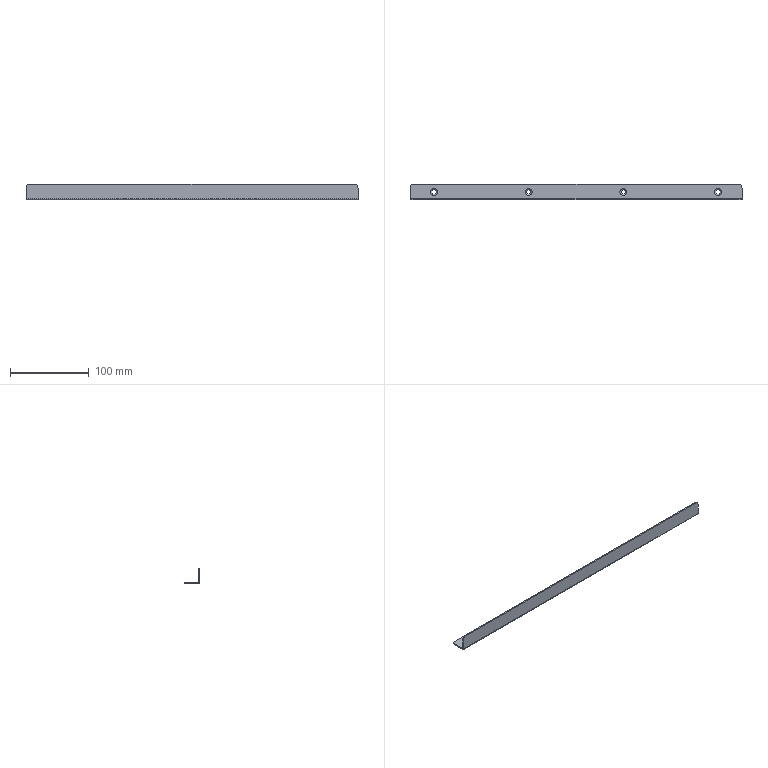Part | SolidWorks | features Chamfer 1, EdgeFlange 1, Fillet 1, FlatPattern 1, ICE 1, LPattern 1, SMBaseFlange 1, SheetMetal 1 | 1 solid | 26 faces | box 421 x 20 x 20 mm | volume 23768 mm3 | plane 12 | cone 8 | cylinder 6 | commonest cylinder face diameters 10 x4 0.4 x1 3.4 x1
STEP:
#1=CARTESIAN_POINT('',(-182.9,0.,-1.5));
#2=VERTEX_POINT('',#1);
#3=CARTESIAN_POINT('',(-177.1,0.,-1.5));
#4=VERTEX_POINT('',#3);
#5=CARTESIAN_POINT('',(-180.,0.,-1.5));
#6=DIRECTION('',(0.,0.,1.));
#7=DIRECTION('',(1.,0.,0.));
#8=AXIS2_PLACEMENT_3D('',#5,#6,#7);
#9=CIRCLE('',#8,2.9);
#10=EDGE_CURVE('',#2,#4,#9,.T.);
#11=ORIENTED_EDGE('',*,*,#10,.F.);
#12=CARTESIAN_POINT('',(-184.4,0.,0.));
#13=VERTEX_POINT('',#12);
#14=CARTESIAN_POINT('',(-182.9,0.,-1.5));
#15=DIRECTION('',(-0.7071,0.,0.7071));
#16=VECTOR('',#15,1000.);
#17=LINE('',#14,#16);
#18=EDGE_CURVE('',#2,#13,#17,.T.);
#19=ORIENTED_EDGE('',*,*,#18,.T.);
#20=CARTESIAN_POINT('',(-175.6,0.,0.));
#21=VERTEX_POINT('',#20);
#22=CARTESIAN_POINT('',(-180.,0.,0.));
#23=DIRECTION('',(0.,0.,-1.));
#24=DIRECTION('',(1.,0.,0.));
#25=AXIS2_PLACEMENT_3D('',#22,#23,#24);
#26=CIRCLE('',#25,4.4);
#27=EDGE_CURVE('',#21,#13,#26,.T.);
#28=ORIENTED_EDGE('',*,*,#27,.F.);
#29=CARTESIAN_POINT('',(-177.1,0.,-1.5));
#30=DIRECTION('',(0.7071,0.,0.7071));
#31=VECTOR('',#30,1000.);
#32=LINE('',#29,#31);
#33=EDGE_CURVE('',#4,#21,#32,.T.);
#34=ORIENTED_EDGE('',*,*,#33,.F.);
#35=EDGE_LOOP('',(#11,#19,#28,#34));
#36=FACE_OUTER_BOUND('',#35,.T.);
#37=CARTESIAN_POINT('',(-180.,0.,-1.5));
#38=DIRECTION('',(0.,0.,1.));
#39=DIRECTION('',(1.,0.,0.));
#40=AXIS2_PLACEMENT_3D('',#37,#38,#39);
#41=CONICAL_SURFACE('',#40,2.9,0.7854);
#42=ADVANCED_FACE('',(#36),#41,.F.);
#43=CARTESIAN_POINT('',(-62.9,0.,-1.5));
#44=VERTEX_POINT('',#43);
#45=CARTESIAN_POINT('',(-57.1,0.,-1.5));
#46=VERTEX_POINT('',#45);
#47=CARTESIAN_POINT('',(-60.,0.,-1.5));
#48=DIRECTION('',(0.,0.,1.));
#49=DIRECTION('',(1.,0.,0.));
#50=AXIS2_PLACEMENT_3D('',#47,#48,#49);
#51=CIRCLE('',#50,2.9);
#52=EDGE_CURVE('',#44,#46,#51,.T.);
#53=ORIENTED_EDGE('',*,*,#52,.F.);
#54=CARTESIAN_POINT('',(-64.4,0.,0.));
#55=VERTEX_POINT('',#54);
#56=CARTESIAN_POINT('',(-62.9,0.,-1.5));
#57=DIRECTION('',(-0.7071,0.,0.7071));
#58=VECTOR('',#57,1000.);
#59=LINE('',#56,#58);
#60=EDGE_CURVE('',#44,#55,#59,.T.);
#61=ORIENTED_EDGE('',*,*,#60,.T.);
#62=CARTESIAN_POINT('',(-55.6,0.,0.));
#63=VERTEX_POINT('',#62);
#64=CARTESIAN_POINT('',(-60.,0.,0.));
#65=DIRECTION('',(0.,0.,-1.));
#66=DIRECTION('',(1.,0.,0.));
#67=AXIS2_PLACEMENT_3D('',#64,#65,#66);
#68=CIRCLE('',#67,4.4);
#69=EDGE_CURVE('',#63,#55,#68,.T.);
#70=ORIENTED_EDGE('',*,*,#69,.F.);
#71=CARTESIAN_POINT('',(-57.1,0.,-1.5));
#72=DIRECTION('',(0.7071,0.,0.7071));
#73=VECTOR('',#72,1000.);
#74=LINE('',#71,#73);
#75=EDGE_CURVE('',#46,#63,#74,.T.);
#76=ORIENTED_EDGE('',*,*,#75,.F.);
#77=EDGE_LOOP('',(#53,#61,#70,#76));
#78=FACE_OUTER_BOUND('',#77,.T.);
#79=CARTESIAN_POINT('',(-60.,0.,-1.5));
#80=DIRECTION('',(0.,0.,1.));
#81=DIRECTION('',(1.,0.,0.));
#82=AXIS2_PLACEMENT_3D('',#79,#80,#81);
#83=CONICAL_SURFACE('',#82,2.9,0.7854);
#84=ADVANCED_FACE('',(#78),#83,.F.);
#85=CARTESIAN_POINT('',(57.1,0.,-1.5));
#86=VERTEX_POINT('',#85);
#87=CARTESIAN_POINT('',(62.9,0.,-1.5));
#88=VERTEX_POINT('',#87);
#89=CARTESIAN_POINT('',(60.,0.,-1.5));
#90=DIRECTION('',(0.,0.,1.));
#91=DIRECTION('',(1.,0.,0.));
#92=AXIS2_PLACEMENT_3D('',#89,#90,#91);
#93=CIRCLE('',#92,2.9);
#94=EDGE_CURVE('',#86,#88,#93,.T.);
#95=ORIENTED_EDGE('',*,*,#94,.F.);
#96=CARTESIAN_POINT('',(55.6,0.,0.));
#97=VERTEX_POINT('',#96);
#98=CARTESIAN_POINT('',(57.1,0.,-1.5));
#99=DIRECTION('',(-0.7071,0.,0.7071));
#100=VECTOR('',#99,1000.);
#101=LINE('',#98,#100);
#102=EDGE_CURVE('',#86,#97,#101,.T.);
#103=ORIENTED_EDGE('',*,*,#102,.T.);
#104=CARTESIAN_POINT('',(64.4,0.,0.));
#105=VERTEX_POINT('',#104);
#106=CARTESIAN_POINT('',(60.,0.,0.));
#107=DIRECTION('',(0.,0.,-1.));
#108=DIRECTION('',(1.,0.,0.));
#109=AXIS2_PLACEMENT_3D('',#106,#107,#108);
#110=CIRCLE('',#109,4.4);
#111=EDGE_CURVE('',#105,#97,#110,.T.);
#112=ORIENTED_EDGE('',*,*,#111,.F.);
#113=CARTESIAN_POINT('',(62.9,0.,-1.5));
#114=DIRECTION('',(0.7071,0.,0.7071));
#115=VECTOR('',#114,1000.);
#116=LINE('',#113,#115);
#117=EDGE_CURVE('',#88,#105,#116,.T.);
#118=ORIENTED_EDGE('',*,*,#117,.F.);
#119=EDGE_LOOP('',(#95,#103,#112,#118));
#120=FACE_OUTER_BOUND('',#119,.T.);
#121=CARTESIAN_POINT('',(60.,0.,-1.5));
#122=DIRECTION('',(0.,0.,1.));
#123=DIRECTION('',(1.,0.,0.));
#124=AXIS2_PLACEMENT_3D('',#121,#122,#123);
#125=CONICAL_SURFACE('',#124,2.9,0.7854);
#126=ADVANCED_FACE('',(#120),#125,.F.);
#127=CARTESIAN_POINT('',(177.1,0.,-1.5));
#128=VERTEX_POINT('',#127);
#129=CARTESIAN_POINT('',(182.9,0.,-1.5));
#130=VERTEX_POINT('',#129);
#131=CARTESIAN_POINT('',(180.,0.,-1.5));
#132=DIRECTION('',(0.,0.,1.));
#133=DIRECTION('',(1.,0.,0.));
#134=AXIS2_PLACEMENT_3D('',#131,#132,#133);
#135=CIRCLE('',#134,2.9);
#136=EDGE_CURVE('',#128,#130,#135,.T.);
#137=ORIENTED_EDGE('',*,*,#136,.F.);
#138=CARTESIAN_POINT('',(175.6,0.,0.));
#139=VERTEX_POINT('',#138);
#140=CARTESIAN_POINT('',(177.1,0.,-1.5));
#141=DIRECTION('',(-0.7071,0.,0.7071));
#142=VECTOR('',#141,1000.);
#143=LINE('',#140,#142);
#144=EDGE_CURVE('',#128,#139,#143,.T.);
#145=ORIENTED_EDGE('',*,*,#144,.T.);
#146=CARTESIAN_POINT('',(184.4,0.,0.));
#147=VERTEX_POINT('',#146);
#148=CARTESIAN_POINT('',(180.,0.,0.));
#149=DIRECTION('',(0.,0.,-1.));
#150=DIRECTION('',(1.,0.,0.));
#151=AXIS2_PLACEMENT_3D('',#148,#149,#150);
#152=CIRCLE('',#151,4.4);
#153=EDGE_CURVE('',#147,#139,#152,.T.);
#154=ORIENTED_EDGE('',*,*,#153,.F.);
#155=CARTESIAN_POINT('',(182.9,0.,-1.5));
#156=DIRECTION('',(0.7071,0.,0.7071));
#157=VECTOR('',#156,1000.);
#158=LINE('',#155,#157);
#159=EDGE_CURVE('',#130,#147,#158,.T.);
#160=ORIENTED_EDGE('',*,*,#159,.F.);
#161=EDGE_LOOP('',(#137,#145,#154,#160));
#162=FACE_OUTER_BOUND('',#161,.T.);
#163=CARTESIAN_POINT('',(180.,0.,-1.5));
#164=DIRECTION('',(0.,0.,1.));
#165=DIRECTION('',(1.,0.,0.));
#166=AXIS2_PLACEMENT_3D('',#163,#164,#165);
#167=CONICAL_SURFACE('',#166,2.9,0.7854);
#168=ADVANCED_FACE('',(#162),#167,.F.);
#169=CARTESIAN_POINT('',(210.5,-8.3,-1.5));
#170=VERTEX_POINT('',#169);
#171=CARTESIAN_POINT('',(210.5,5.,-1.5));
#172=VERTEX_POINT('',#171);
#173=CARTESIAN_POINT('',(210.5,10.,-1.5));
#174=DIRECTION('',(0.,1.,0.));
#175=VECTOR('',#174,1000.);
#176=LINE('',#173,#175);
#177=EDGE_CURVE('',#170,#172,#176,.T.);
#178=ORIENTED_EDGE('',*,*,#177,.T.);
#179=CARTESIAN_POINT('',(210.5,5.,0.));
#180=VERTEX_POINT('',#179);
#181=CARTESIAN_POINT('',(210.5,5.,-1.5));
#182=DIRECTION('',(0.,0.,1.));
#183=VECTOR('',#182,1000.);
#184=LINE('',#181,#183);
#185=EDGE_CURVE('',#172,#180,#184,.T.);
#186=ORIENTED_EDGE('',*,*,#185,.T.);
#187=CARTESIAN_POINT('',(210.5,-8.3,0.));
#188=VERTEX_POINT('',#187);
#189=CARTESIAN_POINT('',(210.5,10.,0.));
#190=DIRECTION('',(0.,1.,0.));
#191=VECTOR('',#190,1000.);
#192=LINE('',#189,#191);
#193=EDGE_CURVE('',#188,#180,#192,.T.);
#194=ORIENTED_EDGE('',*,*,#193,.F.);
#195=CARTESIAN_POINT('',(210.5,-8.3,0.));
#196=DIRECTION('',(0.,0.,-1.));
#197=VECTOR('',#196,1000.);
#198=LINE('',#195,#197);
#199=EDGE_CURVE('',#188,#170,#198,.T.);
#200=ORIENTED_EDGE('',*,*,#199,.T.);
#201=EDGE_LOOP('',(#178,#186,#194,#200));
#202=FACE_OUTER_BOUND('',#201,.T.);
#203=CARTESIAN_POINT('',(210.5,10.,-1.5));
#204=DIRECTION('',(1.,0.,0.));
#205=DIRECTION('',(0.,0.,-1.));
#206=AXIS2_PLACEMENT_3D('',#203,#204,#205);
#207=PLANE('',#206);
#208=ADVANCED_FACE('',(#202),#207,.T.);
#209=CARTESIAN_POINT('',(180.,0.,-1.5));
#210=DIRECTION('',(0.,0.,1.));
#211=DIRECTION('',(1.,0.,0.));
#212=AXIS2_PLACEMENT_3D('',#209,#210,#211);
#213=CIRCLE('',#212,2.9);
#214=EDGE_CURVE('',#130,#128,#213,.T.);
#215=ORIENTED_EDGE('',*,*,#214,.T.);
#216=ORIENTED_EDGE('',*,*,#136,.T.);
#217=EDGE_LOOP('',(#215,#216));
#218=FACE_BOUND('',#217,.T.);
#219=CARTESIAN_POINT('',(60.,0.,-1.5));
#220=DIRECTION('',(0.,0.,1.));
#221=DIRECTION('',(1.,0.,0.));
#222=AXIS2_PLACEMENT_3D('',#219,#220,#221);
#223=CIRCLE('',#222,2.9);
#224=EDGE_CURVE('',#88,#86,#223,.T.);
#225=ORIENTED_EDGE('',*,*,#224,.T.);
#226=ORIENTED_EDGE('',*,*,#94,.T.);
#227=EDGE_LOOP('',(#225,#226));
#228=FACE_BOUND('',#227,.T.);
#229=CARTESIAN_POINT('',(-180.,0.,-1.5));
#230=DIRECTION('',(0.,0.,1.));
#231=DIRECTION('',(1.,0.,0.));
#232=AXIS2_PLACEMENT_3D('',#229,#230,#231);
#233=CIRCLE('',#232,2.9);
#234=EDGE_CURVE('',#4,#2,#233,.T.);
#235=ORIENTED_EDGE('',*,*,#234,.T.);
#236=ORIENTED_EDGE('',*,*,#10,.T.);
#237=EDGE_LOOP('',(#235,#236));
#238=FACE_BOUND('',#237,.T.);
#239=CARTESIAN_POINT('',(-60.,0.,-1.5));
#240=DIRECTION('',(0.,0.,1.));
#241=DIRECTION('',(1.,0.,0.));
#242=AXIS2_PLACEMENT_3D('',#239,#240,#241);
#243=CIRCLE('',#242,2.9);
#244=EDGE_CURVE('',#46,#44,#243,.T.);
#245=ORIENTED_EDGE('',*,*,#244,.T.);
#246=ORIENTED_EDGE('',*,*,#52,.T.);
#247=EDGE_LOOP('',(#245,#246));
#248=FACE_BOUND('',#247,.T.);
#249=CARTESIAN_POINT('',(205.5,10.,-1.5));
#250=VERTEX_POINT('',#249);
#251=CARTESIAN_POINT('',(-205.5,10.,-1.5));
#252=VERTEX_POINT('',#251);
#253=CARTESIAN_POINT('',(-210.5,10.,-1.5));
#254=DIRECTION('',(-1.,0.,0.));
#255=VECTOR('',#254,1000.);
#256=LINE('',#253,#255);
#257=EDGE_CURVE('',#250,#252,#256,.T.);
#258=ORIENTED_EDGE('',*,*,#257,.F.);
#259=CARTESIAN_POINT('',(205.5,5.,-1.5));
#260=DIRECTION('',(0.,0.,-1.));
#261=DIRECTION('',(1.,0.,0.));
#262=AXIS2_PLACEMENT_3D('',#259,#260,#261);
#263=CIRCLE('',#262,5.);
#264=EDGE_CURVE('',#250,#172,#263,.T.);
#265=ORIENTED_EDGE('',*,*,#264,.T.);
#266=ORIENTED_EDGE('',*,*,#177,.F.);
#267=CARTESIAN_POINT('',(-210.5,-8.3,-1.5));
#268=VERTEX_POINT('',#267);
#269=CARTESIAN_POINT('',(210.5,-8.3,-1.5));
#270=DIRECTION('',(-1.,0.,0.));
#271=VECTOR('',#270,1000.);
#272=LINE('',#269,#271);
#273=EDGE_CURVE('',#170,#268,#272,.T.);
#274=ORIENTED_EDGE('',*,*,#273,.T.);
#275=CARTESIAN_POINT('',(-210.5,5.,-1.5));
#276=VERTEX_POINT('',#275);
#277=CARTESIAN_POINT('',(-210.5,10.,-1.5));
#278=DIRECTION('',(0.,-1.,0.));
#279=VECTOR('',#278,1000.);
#280=LINE('',#277,#279);
#281=EDGE_CURVE('',#276,#268,#280,.T.);
#282=ORIENTED_EDGE('',*,*,#281,.F.);
#283=CARTESIAN_POINT('',(-205.5,5.,-1.5));
#284=DIRECTION('',(0.,0.,-1.));
#285=DIRECTION('',(1.,0.,0.));
#286=AXIS2_PLACEMENT_3D('',#283,#284,#285);
#287=CIRCLE('',#286,5.);
#288=EDGE_CURVE('',#276,#252,#287,.T.);
#289=ORIENTED_EDGE('',*,*,#288,.T.);
#290=EDGE_LOOP('',(#258,#265,#266,#274,#282,#289));
#291=FACE_OUTER_BOUND('',#290,.T.);
#292=CARTESIAN_POINT('',(0.,0.,-1.5));
#293=DIRECTION('',(0.,0.,1.));
#294=DIRECTION('',(1.,0.,0.));
#295=AXIS2_PLACEMENT_3D('',#292,#293,#294);
#296=PLANE('',#295);
#297=ADVANCED_FACE('',(#218,#228,#238,#248,#291),#296,.F.);
#298=ORIENTED_EDGE('',*,*,#27,.T.);
#299=CARTESIAN_POINT('',(-180.,0.,0.));
#300=DIRECTION('',(0.,0.,-1.));
#301=DIRECTION('',(1.,0.,0.));
#302=AXIS2_PLACEMENT_3D('',#299,#300,#301);
#303=CIRCLE('',#302,4.4);
#304=EDGE_CURVE('',#13,#21,#303,.T.);
#305=ORIENTED_EDGE('',*,*,#304,.T.);
#306=EDGE_LOOP('',(#298,#305));
#307=FACE_BOUND('',#306,.T.);
#308=ORIENTED_EDGE('',*,*,#69,.T.);
#309=CARTESIAN_POINT('',(-60.,0.,0.));
#310=DIRECTION('',(0.,0.,-1.));
#311=DIRECTION('',(1.,0.,0.));
#312=AXIS2_PLACEMENT_3D('',#309,#310,#311);
#313=CIRCLE('',#312,4.4);
#314=EDGE_CURVE('',#55,#63,#313,.T.);
#315=ORIENTED_EDGE('',*,*,#314,.T.);
#316=EDGE_LOOP('',(#308,#315));
#317=FACE_BOUND('',#316,.T.);
#318=ORIENTED_EDGE('',*,*,#111,.T.);
#319=CARTESIAN_POINT('',(60.,0.,0.));
#320=DIRECTION('',(0.,0.,-1.));
#321=DIRECTION('',(1.,0.,0.));
#322=AXIS2_PLACEMENT_3D('',#319,#320,#321);
#323=CIRCLE('',#322,4.4);
#324=EDGE_CURVE('',#97,#105,#323,.T.);
#325=ORIENTED_EDGE('',*,*,#324,.T.);
#326=EDGE_LOOP('',(#318,#325));
#327=FACE_BOUND('',#326,.T.);
#328=ORIENTED_EDGE('',*,*,#153,.T.);
#329=CARTESIAN_POINT('',(180.,0.,0.));
#330=DIRECTION('',(0.,0.,-1.));
#331=DIRECTION('',(1.,0.,0.));
#332=AXIS2_PLACEMENT_3D('',#329,#330,#331);
#333=CIRCLE('',#332,4.4);
#334=EDGE_CURVE('',#139,#147,#333,.T.);
#335=ORIENTED_EDGE('',*,*,#334,.T.);
#336=EDGE_LOOP('',(#328,#335));
#337=FACE_BOUND('',#336,.T.);
#338=ORIENTED_EDGE('',*,*,#193,.T.);
#339=CARTESIAN_POINT('',(205.5,10.,0.));
#340=VERTEX_POINT('',#339);
#341=CARTESIAN_POINT('',(205.5,5.,0.));
#342=DIRECTION('',(0.,0.,1.));
#343=DIRECTION('',(1.,0.,0.));
#344=AXIS2_PLACEMENT_3D('',#341,#342,#343);
#345=CIRCLE('',#344,5.);
#346=EDGE_CURVE('',#180,#340,#345,.T.);
#347=ORIENTED_EDGE('',*,*,#346,.T.);
#348=CARTESIAN_POINT('',(-205.5,10.,0.));
#349=VERTEX_POINT('',#348);
#350=CARTESIAN_POINT('',(-210.5,10.,0.));
#351=DIRECTION('',(-1.,0.,0.));
#352=VECTOR('',#351,1000.);
#353=LINE('',#350,#352);
#354=EDGE_CURVE('',#340,#349,#353,.T.);
#355=ORIENTED_EDGE('',*,*,#354,.T.);
#356=CARTESIAN_POINT('',(-210.5,5.,0.));
#357=VERTEX_POINT('',#356);
#358=CARTESIAN_POINT('',(-205.5,5.,0.));
#359=DIRECTION('',(0.,0.,1.));
#360=DIRECTION('',(1.,0.,0.));
#361=AXIS2_PLACEMENT_3D('',#358,#359,#360);
#362=CIRCLE('',#361,5.);
#363=EDGE_CURVE('',#349,#357,#362,.T.);
#364=ORIENTED_EDGE('',*,*,#363,.T.);
#365=CARTESIAN_POINT('',(-210.5,-8.3,0.));
#366=VERTEX_POINT('',#365);
#367=CARTESIAN_POINT('',(-210.5,10.,0.));
#368=DIRECTION('',(0.,-1.,0.));
#369=VECTOR('',#368,1000.);
#370=LINE('',#367,#369);
#371=EDGE_CURVE('',#357,#366,#370,.T.);
#372=ORIENTED_EDGE('',*,*,#371,.T.);
#373=CARTESIAN_POINT('',(210.5,-8.3,0.));
#374=DIRECTION('',(-1.,0.,0.));
#375=VECTOR('',#374,1000.);
#376=LINE('',#373,#375);
#377=EDGE_CURVE('',#188,#366,#376,.T.);
#378=ORIENTED_EDGE('',*,*,#377,.F.);
#379=EDGE_LOOP('',(#338,#347,#355,#364,#372,#378));
#380=FACE_OUTER_BOUND('',#379,.T.);
#381=CARTESIAN_POINT('',(0.,0.,0.));
#382=DIRECTION('',(0.,0.,1.));
#383=DIRECTION('',(1.,0.,0.));
#384=AXIS2_PLACEMENT_3D('',#381,#382,#383);
#385=PLANE('',#384);
#386=ADVANCED_FACE('',(#307,#317,#327,#337,#380),#385,.T.);
#387=ORIENTED_EDGE('',*,*,#371,.F.);
#388=CARTESIAN_POINT('',(-210.5,5.,-1.5));
#389=DIRECTION('',(0.,0.,-1.));
#390=VECTOR('',#389,1000.);
#391=LINE('',#388,#390);
#392=EDGE_CURVE('',#357,#276,#391,.T.);
#393=ORIENTED_EDGE('',*,*,#392,.T.);
#394=ORIENTED_EDGE('',*,*,#281,.T.);
#395=CARTESIAN_POINT('',(-210.5,-8.3,0.));
#396=DIRECTION('',(0.,0.,-1.));
#397=VECTOR('',#396,1000.);
#398=LINE('',#395,#397);
#399=EDGE_CURVE('',#366,#268,#398,.T.);
#400=ORIENTED_EDGE('',*,*,#399,.F.);
#401=EDGE_LOOP('',(#387,#393,#394,#400));
#402=FACE_OUTER_BOUND('',#401,.T.);
#403=CARTESIAN_POINT('',(-210.5,10.,-1.5));
#404=DIRECTION('',(-1.,0.,0.));
#405=DIRECTION('',(0.,0.,1.));
#406=AXIS2_PLACEMENT_3D('',#403,#404,#405);
#407=PLANE('',#406);
#408=ADVANCED_FACE('',(#402),#407,.T.);
#409=ORIENTED_EDGE('',*,*,#354,.F.);
#410=CARTESIAN_POINT('',(205.5,10.,-1.5));
#411=DIRECTION('',(0.,0.,-1.));
#412=VECTOR('',#411,1000.);
#413=LINE('',#410,#412);
#414=EDGE_CURVE('',#340,#250,#413,.T.);
#415=ORIENTED_EDGE('',*,*,#414,.T.);
#416=ORIENTED_EDGE('',*,*,#257,.T.);
#417=CARTESIAN_POINT('',(-205.5,10.,-1.5));
#418=DIRECTION('',(0.,0.,1.));
#419=VECTOR('',#418,1000.);
#420=LINE('',#417,#419);
#421=EDGE_CURVE('',#252,#349,#420,.T.);
#422=ORIENTED_EDGE('',*,*,#421,.T.);
#423=EDGE_LOOP('',(#409,#415,#416,#422));
#424=FACE_OUTER_BOUND('',#423,.T.);
#425=CARTESIAN_POINT('',(-210.5,10.,-1.5));
#426=DIRECTION('',(0.,1.,0.));
#427=DIRECTION('',(0.,0.,1.));
#428=AXIS2_PLACEMENT_3D('',#425,#426,#427);
#429=PLANE('',#428);
#430=ADVANCED_FACE('',(#424),#429,.T.);
#431=ORIENTED_EDGE('',*,*,#144,.F.);
#432=ORIENTED_EDGE('',*,*,#214,.F.);
#433=ORIENTED_EDGE('',*,*,#159,.T.);
#434=ORIENTED_EDGE('',*,*,#334,.F.);
#435=EDGE_LOOP('',(#431,#432,#433,#434));
#436=FACE_OUTER_BOUND('',#435,.T.);
#437=CARTESIAN_POINT('',(180.,0.,-1.5));
#438=DIRECTION('',(0.,0.,1.));
#439=DIRECTION('',(1.,0.,0.));
#440=AXIS2_PLACEMENT_3D('',#437,#438,#439);
#441=CONICAL_SURFACE('',#440,2.9,0.7854);
#442=ADVANCED_FACE('',(#436),#441,.F.);
#443=ORIENTED_EDGE('',*,*,#102,.F.);
#444=ORIENTED_EDGE('',*,*,#224,.F.);
#445=ORIENTED_EDGE('',*,*,#117,.T.);
#446=ORIENTED_EDGE('',*,*,#324,.F.);
#447=EDGE_LOOP('',(#443,#444,#445,#446));
#448=FACE_OUTER_BOUND('',#447,.T.);
#449=CARTESIAN_POINT('',(60.,0.,-1.5));
#450=DIRECTION('',(0.,0.,1.));
#451=DIRECTION('',(1.,0.,0.));
#452=AXIS2_PLACEMENT_3D('',#449,#450,#451);
#453=CONICAL_SURFACE('',#452,2.9,0.7854);
#454=ADVANCED_FACE('',(#448),#453,.F.);
#455=ORIENTED_EDGE('',*,*,#60,.F.);
#456=ORIENTED_EDGE('',*,*,#244,.F.);
#457=ORIENTED_EDGE('',*,*,#75,.T.);
#458=ORIENTED_EDGE('',*,*,#314,.F.);
#459=EDGE_LOOP('',(#455,#456,#457,#458));
#460=FACE_OUTER_BOUND('',#459,.T.);
#461=CARTESIAN_POINT('',(-60.,0.,-1.5));
#462=DIRECTION('',(0.,0.,1.));
#463=DIRECTION('',(1.,0.,0.));
#464=AXIS2_PLACEMENT_3D('',#461,#462,#463);
#465=CONICAL_SURFACE('',#464,2.9,0.7854);
#466=ADVANCED_FACE('',(#460),#465,.F.);
#467=ORIENTED_EDGE('',*,*,#18,.F.);
#468=ORIENTED_EDGE('',*,*,#234,.F.);
#469=ORIENTED_EDGE('',*,*,#33,.T.);
#470=ORIENTED_EDGE('',*,*,#304,.F.);
#471=EDGE_LOOP('',(#467,#468,#469,#470));
#472=FACE_OUTER_BOUND('',#471,.T.);
#473=CARTESIAN_POINT('',(-180.,0.,-1.5));
#474=DIRECTION('',(0.,0.,1.));
#475=DIRECTION('',(1.,0.,0.));
#476=AXIS2_PLACEMENT_3D('',#473,#474,#475);
#477=CONICAL_SURFACE('',#476,2.9,0.7854);
#478=ADVANCED_FACE('',(#472),#477,.F.);
#479=CARTESIAN_POINT('',(-210.5,-8.5,0.2));
#480=VERTEX_POINT('',#479);
#481=CARTESIAN_POINT('',(-210.5,-10.,0.2));
#482=VERTEX_POINT('',#481);
#483=CARTESIAN_POINT('',(-210.5,-10.,0.2));
#484=DIRECTION('',(0.,-1.,0.));
#485=VECTOR('',#484,1000.);
#486=LINE('',#483,#485);
#487=EDGE_CURVE('',#480,#482,#486,.T.);
#488=ORIENTED_EDGE('',*,*,#487,.F.);
#489=CARTESIAN_POINT('',(-210.5,-8.3,0.2));
#490=DIRECTION('',(-1.,0.,0.));
#491=DIRECTION('',(0.,0.,-1.));
#492=AXIS2_PLACEMENT_3D('',#489,#490,#491);
#493=CIRCLE('',#492,0.2);
#494=EDGE_CURVE('',#366,#480,#493,.T.);
#495=ORIENTED_EDGE('',*,*,#494,.F.);
#496=ORIENTED_EDGE('',*,*,#399,.T.);
#497=CARTESIAN_POINT('',(-210.5,-8.3,0.2));
#498=DIRECTION('',(-1.,0.,0.));
#499=DIRECTION('',(0.,0.,-1.));
#500=AXIS2_PLACEMENT_3D('',#497,#498,#499);
#501=CIRCLE('',#500,1.7);
#502=EDGE_CURVE('',#268,#482,#501,.T.);
#503=ORIENTED_EDGE('',*,*,#502,.T.);
#504=EDGE_LOOP('',(#488,#495,#496,#503));
#505=FACE_OUTER_BOUND('',#504,.T.);
#506=CARTESIAN_POINT('',(-210.5,-8.3,0.2));
#507=DIRECTION('',(-1.,0.,0.));
#508=DIRECTION('',(0.,0.,1.));
#509=AXIS2_PLACEMENT_3D('',#506,#507,#508);
#510=PLANE('',#509);
#511=ADVANCED_FACE('',(#505),#510,.T.);
#512=CARTESIAN_POINT('',(210.5,-8.5,0.2));
#513=VERTEX_POINT('',#512);
#514=CARTESIAN_POINT('',(210.5,-8.3,0.2));
#515=DIRECTION('',(1.,0.,0.));
#516=DIRECTION('',(0.,0.,-1.));
#517=AXIS2_PLACEMENT_3D('',#514,#515,#516);
#518=CIRCLE('',#517,0.2);
#519=EDGE_CURVE('',#513,#188,#518,.T.);
#520=ORIENTED_EDGE('',*,*,#519,.F.);
#521=CARTESIAN_POINT('',(210.5,-10.,0.2));
#522=VERTEX_POINT('',#521);
#523=CARTESIAN_POINT('',(210.5,-8.5,0.2));
#524=DIRECTION('',(0.,-1.,0.));
#525=VECTOR('',#524,1000.);
#526=LINE('',#523,#525);
#527=EDGE_CURVE('',#513,#522,#526,.T.);
#528=ORIENTED_EDGE('',*,*,#527,.T.);
#529=CARTESIAN_POINT('',(210.5,-8.3,0.2));
#530=DIRECTION('',(1.,0.,0.));
#531=DIRECTION('',(0.,0.,-1.));
#532=AXIS2_PLACEMENT_3D('',#529,#530,#531);
#533=CIRCLE('',#532,1.7);
#534=EDGE_CURVE('',#522,#170,#533,.T.);
#535=ORIENTED_EDGE('',*,*,#534,.T.);
#536=ORIENTED_EDGE('',*,*,#199,.F.);
#537=EDGE_LOOP('',(#520,#528,#535,#536));
#538=FACE_OUTER_BOUND('',#537,.T.);
#539=CARTESIAN_POINT('',(210.5,-8.3,0.2));
#540=DIRECTION('',(-1.,0.,0.));
#541=DIRECTION('',(0.,0.,1.));
#542=AXIS2_PLACEMENT_3D('',#539,#540,#541);
#543=PLANE('',#542);
#544=ADVANCED_FACE('',(#538),#543,.F.);
#545=ORIENTED_EDGE('',*,*,#273,.F.);
#546=ORIENTED_EDGE('',*,*,#534,.F.);
#547=CARTESIAN_POINT('',(0.,-10.,0.2));
#548=DIRECTION('',(1.,0.,0.));
#549=VECTOR('',#548,1000.);
#550=LINE('',#547,#549);
#551=EDGE_CURVE('',#482,#522,#550,.T.);
#552=ORIENTED_EDGE('',*,*,#551,.F.);
#553=ORIENTED_EDGE('',*,*,#502,.F.);
#554=EDGE_LOOP('',(#545,#546,#552,#553));
#555=FACE_OUTER_BOUND('',#554,.T.);
#556=CARTESIAN_POINT('',(210.5,-8.3,0.2));
#557=DIRECTION('',(1.,0.,0.));
#558=DIRECTION('',(0.,-1.,0.));
#559=AXIS2_PLACEMENT_3D('',#556,#557,#558);
#560=CYLINDRICAL_SURFACE('',#559,1.7);
#561=ADVANCED_FACE('',(#555),#560,.T.);
#562=ORIENTED_EDGE('',*,*,#377,.T.);
#563=ORIENTED_EDGE('',*,*,#494,.T.);
#564=CARTESIAN_POINT('',(-210.5,-8.5,0.2));
#565=DIRECTION('',(1.,0.,0.));
#566=VECTOR('',#565,1000.);
#567=LINE('',#564,#566);
#568=EDGE_CURVE('',#480,#513,#567,.T.);
#569=ORIENTED_EDGE('',*,*,#568,.T.);
#570=ORIENTED_EDGE('',*,*,#519,.T.);
#571=EDGE_LOOP('',(#562,#563,#569,#570));
#572=FACE_OUTER_BOUND('',#571,.T.);
#573=CARTESIAN_POINT('',(210.5,-8.3,0.2));
#574=DIRECTION('',(1.,0.,0.));
#575=DIRECTION('',(0.,-1.,0.));
#576=AXIS2_PLACEMENT_3D('',#573,#574,#575);
#577=CYLINDRICAL_SURFACE('',#576,0.2);
#578=ADVANCED_FACE('',(#572),#577,.F.);
#579=CARTESIAN_POINT('',(210.5,-8.5,13.5));
#580=VERTEX_POINT('',#579);
#581=CARTESIAN_POINT('',(210.5,-8.5,0.));
#582=DIRECTION('',(0.,0.,-1.));
#583=VECTOR('',#582,1000.);
#584=LINE('',#581,#583);
#585=EDGE_CURVE('',#580,#513,#584,.T.);
#586=ORIENTED_EDGE('',*,*,#585,.F.);
#587=CARTESIAN_POINT('',(210.5,-10.,13.5));
#588=VERTEX_POINT('',#587);
#589=CARTESIAN_POINT('',(210.5,-10.,13.5));
#590=DIRECTION('',(0.,-1.,0.));
#591=VECTOR('',#590,1000.);
#592=LINE('',#589,#591);
#593=EDGE_CURVE('',#580,#588,#592,.T.);
#594=ORIENTED_EDGE('',*,*,#593,.T.);
#595=CARTESIAN_POINT('',(210.5,-10.,0.));
#596=DIRECTION('',(0.,0.,-1.));
#597=VECTOR('',#596,1000.);
#598=LINE('',#595,#597);
#599=EDGE_CURVE('',#588,#522,#598,.T.);
#600=ORIENTED_EDGE('',*,*,#599,.T.);
#601=ORIENTED_EDGE('',*,*,#527,.F.);
#602=EDGE_LOOP('',(#586,#594,#600,#601));
#603=FACE_OUTER_BOUND('',#602,.T.);
#604=CARTESIAN_POINT('',(210.5,-10.,0.));
#605=DIRECTION('',(1.,0.,0.));
#606=DIRECTION('',(0.,0.,-1.));
#607=AXIS2_PLACEMENT_3D('',#604,#605,#606);
#608=PLANE('',#607);
#609=ADVANCED_FACE('',(#603),#608,.T.);
#610=CARTESIAN_POINT('',(-210.5,-10.,13.5));
#611=VERTEX_POINT('',#610);
#612=CARTESIAN_POINT('',(-210.5,-10.,18.5));
#613=DIRECTION('',(0.,0.,1.));
#614=VECTOR('',#613,1000.);
#615=LINE('',#612,#614);
#616=EDGE_CURVE('',#482,#611,#615,.T.);
#617=ORIENTED_EDGE('',*,*,#616,.T.);
#618=CARTESIAN_POINT('',(-210.5,-8.5,13.5));
#619=VERTEX_POINT('',#618);
#620=CARTESIAN_POINT('',(-210.5,-10.,13.5));
#621=DIRECTION('',(0.,1.,0.));
#622=VECTOR('',#621,1000.);
#623=LINE('',#620,#622);
#624=EDGE_CURVE('',#611,#619,#623,.T.);
#625=ORIENTED_EDGE('',*,*,#624,.T.);
#626=CARTESIAN_POINT('',(-210.5,-8.5,0.));
#627=DIRECTION('',(0.,0.,1.));
#628=VECTOR('',#627,1000.);
#629=LINE('',#626,#628);
#630=EDGE_CURVE('',#480,#619,#629,.T.);
#631=ORIENTED_EDGE('',*,*,#630,.F.);
#632=ORIENTED_EDGE('',*,*,#487,.T.);
#633=EDGE_LOOP('',(#617,#625,#631,#632));
#634=FACE_OUTER_BOUND('',#633,.T.);
#635=CARTESIAN_POINT('',(-210.5,-10.,18.5));
#636=DIRECTION('',(-1.,0.,0.));
#637=DIRECTION('',(0.,0.,1.));
#638=AXIS2_PLACEMENT_3D('',#635,#636,#637);
#639=PLANE('',#638);
#640=ADVANCED_FACE('',(#634),#639,.T.);
#641=ORIENTED_EDGE('',*,*,#599,.F.);
#642=CARTESIAN_POINT('',(205.5,-10.,18.5));
#643=VERTEX_POINT('',#642);
#644=CARTESIAN_POINT('',(205.5,-10.,13.5));
#645=DIRECTION('',(0.,-1.,0.));
#646=DIRECTION('',(0.,0.,-1.));
#647=AXIS2_PLACEMENT_3D('',#644,#645,#646);
#648=CIRCLE('',#647,5.);
#649=EDGE_CURVE('',#588,#643,#648,.T.);
#650=ORIENTED_EDGE('',*,*,#649,.T.);
#651=CARTESIAN_POINT('',(-205.5,-10.,18.5));
#652=VERTEX_POINT('',#651);
#653=CARTESIAN_POINT('',(210.5,-10.,18.5));
#654=DIRECTION('',(1.,0.,0.));
#655=VECTOR('',#654,1000.);
#656=LINE('',#653,#655);
#657=EDGE_CURVE('',#652,#643,#656,.T.);
#658=ORIENTED_EDGE('',*,*,#657,.F.);
#659=CARTESIAN_POINT('',(-205.5,-10.,13.5));
#660=DIRECTION('',(0.,-1.,0.));
#661=DIRECTION('',(0.,0.,-1.));
#662=AXIS2_PLACEMENT_3D('',#659,#660,#661);
#663=CIRCLE('',#662,5.);
#664=EDGE_CURVE('',#652,#611,#663,.T.);
#665=ORIENTED_EDGE('',*,*,#664,.T.);
#666=ORIENTED_EDGE('',*,*,#616,.F.);
#667=ORIENTED_EDGE('',*,*,#551,.T.);
#668=EDGE_LOOP('',(#641,#650,#658,#665,#666,#667));
#669=FACE_OUTER_BOUND('',#668,.T.);
#670=CARTESIAN_POINT('',(0.,-10.,0.));
#671=DIRECTION('',(0.,-1.,0.));
#672=DIRECTION('',(0.,0.,-1.));
#673=AXIS2_PLACEMENT_3D('',#670,#671,#672);
#674=PLANE('',#673);
#675=ADVANCED_FACE('',(#669),#674,.T.);
#676=CARTESIAN_POINT('',(-205.5,-8.5,18.5));
#677=VERTEX_POINT('',#676);
#678=CARTESIAN_POINT('',(205.5,-8.5,18.5));
#679=VERTEX_POINT('',#678);
#680=CARTESIAN_POINT('',(0.,-8.5,18.5));
#681=DIRECTION('',(1.,0.,0.));
#682=VECTOR('',#681,1000.);
#683=LINE('',#680,#682);
#684=EDGE_CURVE('',#677,#679,#683,.T.);
#685=ORIENTED_EDGE('',*,*,#684,.T.);
#686=CARTESIAN_POINT('',(205.5,-8.5,13.5));
#687=DIRECTION('',(0.,1.,0.));
#688=DIRECTION('',(0.,0.,-1.));
#689=AXIS2_PLACEMENT_3D('',#686,#687,#688);
#690=CIRCLE('',#689,5.);
#691=EDGE_CURVE('',#679,#580,#690,.T.);
#692=ORIENTED_EDGE('',*,*,#691,.T.);
#693=ORIENTED_EDGE('',*,*,#585,.T.);
#694=ORIENTED_EDGE('',*,*,#568,.F.);
#695=ORIENTED_EDGE('',*,*,#630,.T.);
#696=CARTESIAN_POINT('',(-205.5,-8.5,13.5));
#697=DIRECTION('',(0.,1.,0.));
#698=DIRECTION('',(0.,0.,-1.));
#699=AXIS2_PLACEMENT_3D('',#696,#697,#698);
#700=CIRCLE('',#699,5.);
#701=EDGE_CURVE('',#619,#677,#700,.T.);
#702=ORIENTED_EDGE('',*,*,#701,.T.);
#703=EDGE_LOOP('',(#685,#692,#693,#694,#695,#702));
#704=FACE_OUTER_BOUND('',#703,.T.);
#705=CARTESIAN_POINT('',(0.,-8.5,0.));
#706=DIRECTION('',(0.,-1.,0.));
#707=DIRECTION('',(0.,0.,-1.));
#708=AXIS2_PLACEMENT_3D('',#705,#706,#707);
#709=PLANE('',#708);
#710=ADVANCED_FACE('',(#704),#709,.F.);
#711=ORIENTED_EDGE('',*,*,#657,.T.);
#712=CARTESIAN_POINT('',(205.5,-10.,18.5));
#713=DIRECTION('',(0.,1.,0.));
#714=VECTOR('',#713,1000.);
#715=LINE('',#712,#714);
#716=EDGE_CURVE('',#643,#679,#715,.T.);
#717=ORIENTED_EDGE('',*,*,#716,.T.);
#718=ORIENTED_EDGE('',*,*,#684,.F.);
#719=CARTESIAN_POINT('',(-205.5,-10.,18.5));
#720=DIRECTION('',(0.,-1.,0.));
#721=VECTOR('',#720,1000.);
#722=LINE('',#719,#721);
#723=EDGE_CURVE('',#677,#652,#722,.T.);
#724=ORIENTED_EDGE('',*,*,#723,.T.);
#725=EDGE_LOOP('',(#711,#717,#718,#724));
#726=FACE_OUTER_BOUND('',#725,.T.);
#727=CARTESIAN_POINT('',(210.5,-10.,18.5));
#728=DIRECTION('',(0.,0.,1.));
#729=DIRECTION('',(0.,-1.,0.));
#730=AXIS2_PLACEMENT_3D('',#727,#728,#729);
#731=PLANE('',#730);
#732=ADVANCED_FACE('',(#726),#731,.T.);
#733=ORIENTED_EDGE('',*,*,#264,.F.);
#734=ORIENTED_EDGE('',*,*,#414,.F.);
#735=ORIENTED_EDGE('',*,*,#346,.F.);
#736=ORIENTED_EDGE('',*,*,#185,.F.);
#737=EDGE_LOOP('',(#733,#734,#735,#736));
#738=FACE_OUTER_BOUND('',#737,.T.);
#739=CARTESIAN_POINT('',(205.5,5.,-1.5));
#740=DIRECTION('',(0.,0.,1.));
#741=DIRECTION('',(1.,0.,0.));
#742=AXIS2_PLACEMENT_3D('',#739,#740,#741);
#743=CYLINDRICAL_SURFACE('',#742,5.);
#744=ADVANCED_FACE('',(#738),#743,.T.);
#745=ORIENTED_EDGE('',*,*,#649,.F.);
#746=ORIENTED_EDGE('',*,*,#593,.F.);
#747=ORIENTED_EDGE('',*,*,#691,.F.);
#748=ORIENTED_EDGE('',*,*,#716,.F.);
#749=EDGE_LOOP('',(#745,#746,#747,#748));
#750=FACE_OUTER_BOUND('',#749,.T.);
#751=CARTESIAN_POINT('',(205.5,-10.,13.5));
#752=DIRECTION('',(0.,1.,0.));
#753=DIRECTION('',(0.,0.,1.));
#754=AXIS2_PLACEMENT_3D('',#751,#752,#753);
#755=CYLINDRICAL_SURFACE('',#754,5.);
#756=ADVANCED_FACE('',(#750),#755,.T.);
#757=ORIENTED_EDGE('',*,*,#288,.F.);
#758=ORIENTED_EDGE('',*,*,#392,.F.);
#759=ORIENTED_EDGE('',*,*,#363,.F.);
#760=ORIENTED_EDGE('',*,*,#421,.F.);
#761=EDGE_LOOP('',(#757,#758,#759,#760));
#762=FACE_OUTER_BOUND('',#761,.T.);
#763=CARTESIAN_POINT('',(-205.5,5.,-1.5));
#764=DIRECTION('',(0.,0.,1.));
#765=DIRECTION('',(1.,0.,0.));
#766=AXIS2_PLACEMENT_3D('',#763,#764,#765);
#767=CYLINDRICAL_SURFACE('',#766,5.);
#768=ADVANCED_FACE('',(#762),#767,.T.);
#769=ORIENTED_EDGE('',*,*,#664,.F.);
#770=ORIENTED_EDGE('',*,*,#723,.F.);
#771=ORIENTED_EDGE('',*,*,#701,.F.);
#772=ORIENTED_EDGE('',*,*,#624,.F.);
#773=EDGE_LOOP('',(#769,#770,#771,#772));
#774=FACE_OUTER_BOUND('',#773,.T.);
#775=CARTESIAN_POINT('',(-205.5,-10.,13.5));
#776=DIRECTION('',(0.,1.,0.));
#777=DIRECTION('',(0.,0.,1.));
#778=AXIS2_PLACEMENT_3D('',#775,#776,#777);
#779=CYLINDRICAL_SURFACE('',#778,5.);
#780=ADVANCED_FACE('',(#774),#779,.T.);
#781=CLOSED_SHELL('',(#42,#84,#126,#168,#208,#297,#386,#408,#430,#442,#454,#466,#478,#511,#544,#561,#578,#609,#640,#675,#710,#732,#744,#756,#768,#780));
#782=MANIFOLD_SOLID_BREP('',#781);
#783=CARTESIAN_POINT('',(0.,0.,0.));
#784=DIRECTION('',(0.,0.,1.));
#785=DIRECTION('',(1.,0.,0.));
#786=AXIS2_PLACEMENT_3D('',#783,#784,#785);
#787=(LENGTH_UNIT()NAMED_UNIT(*)SI_UNIT(.MILLI.,.METRE.));
#788=UNCERTAINTY_MEASURE_WITH_UNIT(LENGTH_MEASURE(0.00001),#787,'','');
#789=(NAMED_UNIT(*)PLANE_ANGLE_UNIT()SI_UNIT($,.RADIAN.));
#790=(NAMED_UNIT(*)SI_UNIT($,.STERADIAN.)SOLID_ANGLE_UNIT());
#791=(GEOMETRIC_REPRESENTATION_CONTEXT(3)GLOBAL_UNCERTAINTY_ASSIGNED_CONTEXT((#788))GLOBAL_UNIT_ASSIGNED_CONTEXT((#787,#789,#790))REPRESENTATION_CONTEXT('',''));
#792=ADVANCED_BREP_SHAPE_REPRESENTATION('',(#782,#786),#791);